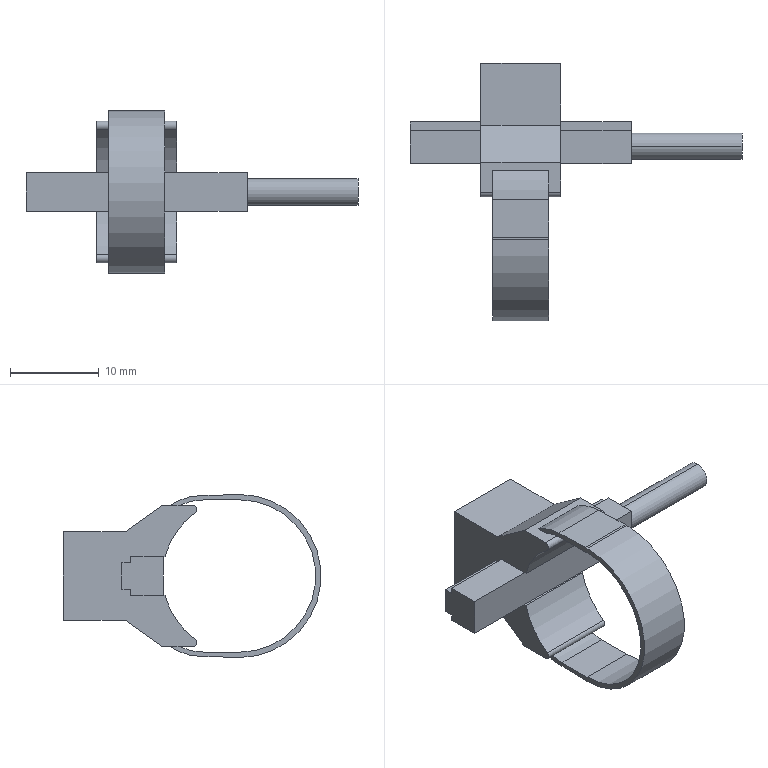Part | SolidWorks | features BaseBody 1 | 1 solid | 49 faces | box 37.5 x 29.1 x 18.4 mm | volume 1877 mm3 | plane 35 | cylinder 14 | commonest cylinder face diameters 12.4 x4 18.4 x3 1 x2 3 x2 17.4 x2 17.2 x1
STEP:
#1=CARTESIAN_POINT('',(24.,10.55,-1.5));
#2=VERTEX_POINT('',#1);
#3=CARTESIAN_POINT('',(24.,10.55,1.5));
#4=VERTEX_POINT('',#3);
#5=CARTESIAN_POINT('',(24.,10.55,0.));
#6=DIRECTION('',(-1.,0.,0.));
#7=DIRECTION('',(0.,0.,-1.));
#8=AXIS2_PLACEMENT_3D('',#5,#6,#7);
#9=CIRCLE('',#8,1.5);
#10=EDGE_CURVE('',#2,#4,#9,.T.);
#11=ORIENTED_EDGE('',*,*,#10,.F.);
#12=CARTESIAN_POINT('',(36.5,10.55,-1.5));
#13=VERTEX_POINT('',#12);
#14=CARTESIAN_POINT('',(36.5,10.55,-1.5));
#15=DIRECTION('',(1.,0.,0.));
#16=VECTOR('',#15,1000.);
#17=LINE('',#14,#16);
#18=EDGE_CURVE('',#2,#13,#17,.T.);
#19=ORIENTED_EDGE('',*,*,#18,.T.);
#20=CARTESIAN_POINT('',(36.5,10.55,1.5));
#21=VERTEX_POINT('',#20);
#22=CARTESIAN_POINT('',(36.5,10.55,0.));
#23=DIRECTION('',(1.,0.,0.));
#24=DIRECTION('',(0.,0.,-1.));
#25=AXIS2_PLACEMENT_3D('',#22,#23,#24);
#26=CIRCLE('',#25,1.5);
#27=EDGE_CURVE('',#21,#13,#26,.T.);
#28=ORIENTED_EDGE('',*,*,#27,.F.);
#29=CARTESIAN_POINT('',(36.5,10.55,1.5));
#30=DIRECTION('',(1.,0.,0.));
#31=VECTOR('',#30,1000.);
#32=LINE('',#29,#31);
#33=EDGE_CURVE('',#4,#21,#32,.T.);
#34=ORIENTED_EDGE('',*,*,#33,.F.);
#35=EDGE_LOOP('',(#11,#19,#28,#34));
#36=FACE_OUTER_BOUND('',#35,.T.);
#37=CARTESIAN_POINT('',(36.5,10.55,0.));
#38=DIRECTION('',(1.,0.,0.));
#39=DIRECTION('',(0.,0.,1.));
#40=AXIS2_PLACEMENT_3D('',#37,#38,#39);
#41=CYLINDRICAL_SURFACE('',#40,1.5);
#42=ADVANCED_FACE('',(#36),#41,.T.);
#43=CARTESIAN_POINT('',(8.325,0.,9.2));
#44=VERTEX_POINT('',#43);
#45=CARTESIAN_POINT('',(8.325,0.,-9.2));
#46=VERTEX_POINT('',#45);
#47=CARTESIAN_POINT('',(8.325,0.,0.));
#48=DIRECTION('',(1.,0.,0.));
#49=DIRECTION('',(0.,0.,-1.));
#50=AXIS2_PLACEMENT_3D('',#47,#48,#49);
#51=CIRCLE('',#50,9.2);
#52=EDGE_CURVE('',#44,#46,#51,.T.);
#53=ORIENTED_EDGE('',*,*,#52,.T.);
#54=CARTESIAN_POINT('',(14.675,0.,-9.2));
#55=VERTEX_POINT('',#54);
#56=CARTESIAN_POINT('',(14.675,0.,-9.2));
#57=DIRECTION('',(1.,0.,0.));
#58=VECTOR('',#57,1000.);
#59=LINE('',#56,#58);
#60=EDGE_CURVE('',#46,#55,#59,.T.);
#61=ORIENTED_EDGE('',*,*,#60,.T.);
#62=CARTESIAN_POINT('',(14.675,0.,9.2));
#63=VERTEX_POINT('',#62);
#64=CARTESIAN_POINT('',(14.675,0.,0.));
#65=DIRECTION('',(1.,0.,0.));
#66=DIRECTION('',(0.,0.,-1.));
#67=AXIS2_PLACEMENT_3D('',#64,#65,#66);
#68=CIRCLE('',#67,9.2);
#69=EDGE_CURVE('',#63,#55,#68,.T.);
#70=ORIENTED_EDGE('',*,*,#69,.F.);
#71=CARTESIAN_POINT('',(14.675,0.,9.2));
#72=DIRECTION('',(1.,0.,0.));
#73=VECTOR('',#72,1000.);
#74=LINE('',#71,#73);
#75=EDGE_CURVE('',#44,#63,#74,.T.);
#76=ORIENTED_EDGE('',*,*,#75,.F.);
#77=EDGE_LOOP('',(#53,#61,#70,#76));
#78=FACE_OUTER_BOUND('',#77,.T.);
#79=CARTESIAN_POINT('',(14.675,0.,0.));
#80=DIRECTION('',(1.,0.,0.));
#81=DIRECTION('',(0.,0.,1.));
#82=AXIS2_PLACEMENT_3D('',#79,#80,#81);
#83=CYLINDRICAL_SURFACE('',#82,9.2);
#84=ADVANCED_FACE('',(#78),#83,.T.);
#85=CARTESIAN_POINT('',(8.325,0.2661,9.196));
#86=VERTEX_POINT('',#85);
#87=CARTESIAN_POINT('',(8.325,0.,0.));
#88=DIRECTION('',(1.,0.,0.));
#89=DIRECTION('',(0.,0.,-1.));
#90=AXIS2_PLACEMENT_3D('',#87,#88,#89);
#91=CIRCLE('',#90,9.2);
#92=EDGE_CURVE('',#86,#44,#91,.T.);
#93=ORIENTED_EDGE('',*,*,#92,.T.);
#94=ORIENTED_EDGE('',*,*,#75,.T.);
#95=CARTESIAN_POINT('',(14.675,0.2661,9.196));
#96=VERTEX_POINT('',#95);
#97=CARTESIAN_POINT('',(14.675,0.,0.));
#98=DIRECTION('',(1.,0.,0.));
#99=DIRECTION('',(0.,0.,-1.));
#100=AXIS2_PLACEMENT_3D('',#97,#98,#99);
#101=CIRCLE('',#100,9.2);
#102=EDGE_CURVE('',#96,#63,#101,.T.);
#103=ORIENTED_EDGE('',*,*,#102,.F.);
#104=CARTESIAN_POINT('',(14.675,0.2661,9.196));
#105=DIRECTION('',(-1.,0.,0.));
#106=VECTOR('',#105,1000.);
#107=LINE('',#104,#106);
#108=EDGE_CURVE('',#96,#86,#107,.T.);
#109=ORIENTED_EDGE('',*,*,#108,.T.);
#110=EDGE_LOOP('',(#93,#94,#103,#109));
#111=FACE_OUTER_BOUND('',#110,.T.);
#112=CARTESIAN_POINT('',(14.675,0.,0.));
#113=DIRECTION('',(1.,0.,0.));
#114=DIRECTION('',(0.,0.,1.));
#115=AXIS2_PLACEMENT_3D('',#112,#113,#114);
#116=CYLINDRICAL_SURFACE('',#115,9.2);
#117=ADVANCED_FACE('',(#111),#116,.T.);
#118=CARTESIAN_POINT('',(7.,19.9,5.));
#119=VERTEX_POINT('',#118);
#120=CARTESIAN_POINT('',(7.,12.9,5.));
#121=VERTEX_POINT('',#120);
#122=CARTESIAN_POINT('',(7.,19.9,5.));
#123=DIRECTION('',(0.,-1.,0.));
#124=VECTOR('',#123,1000.);
#125=LINE('',#122,#124);
#126=EDGE_CURVE('',#119,#121,#125,.T.);
#127=ORIENTED_EDGE('',*,*,#126,.T.);
#128=CARTESIAN_POINT('',(16.,12.9,5.));
#129=VERTEX_POINT('',#128);
#130=CARTESIAN_POINT('',(16.,12.9,5.));
#131=DIRECTION('',(-1.,0.,0.));
#132=VECTOR('',#131,1000.);
#133=LINE('',#130,#132);
#134=EDGE_CURVE('',#129,#121,#133,.T.);
#135=ORIENTED_EDGE('',*,*,#134,.F.);
#136=CARTESIAN_POINT('',(16.,19.9,5.));
#137=VERTEX_POINT('',#136);
#138=CARTESIAN_POINT('',(16.,19.9,5.));
#139=DIRECTION('',(0.,-1.,0.));
#140=VECTOR('',#139,1000.);
#141=LINE('',#138,#140);
#142=EDGE_CURVE('',#137,#129,#141,.T.);
#143=ORIENTED_EDGE('',*,*,#142,.F.);
#144=CARTESIAN_POINT('',(16.,19.9,5.));
#145=DIRECTION('',(-1.,0.,0.));
#146=VECTOR('',#145,1000.);
#147=LINE('',#144,#146);
#148=EDGE_CURVE('',#137,#119,#147,.T.);
#149=ORIENTED_EDGE('',*,*,#148,.T.);
#150=EDGE_LOOP('',(#127,#135,#143,#149));
#151=FACE_OUTER_BOUND('',#150,.T.);
#152=CARTESIAN_POINT('',(16.,19.9,5.));
#153=DIRECTION('',(0.,0.,-1.));
#154=DIRECTION('',(0.,-1.,0.));
#155=AXIS2_PLACEMENT_3D('',#152,#153,#154);
#156=PLANE('',#155);
#157=ADVANCED_FACE('',(#151),#156,.F.);
#158=CARTESIAN_POINT('',(7.,19.9,-5.));
#159=VERTEX_POINT('',#158);
#160=CARTESIAN_POINT('',(7.,19.9,-5.));
#161=DIRECTION('',(0.,0.,1.));
#162=VECTOR('',#161,1000.);
#163=LINE('',#160,#162);
#164=EDGE_CURVE('',#159,#119,#163,.T.);
#165=ORIENTED_EDGE('',*,*,#164,.T.);
#166=ORIENTED_EDGE('',*,*,#148,.F.);
#167=CARTESIAN_POINT('',(16.,19.9,-5.));
#168=VERTEX_POINT('',#167);
#169=CARTESIAN_POINT('',(16.,19.9,-5.));
#170=DIRECTION('',(0.,0.,1.));
#171=VECTOR('',#170,1000.);
#172=LINE('',#169,#171);
#173=EDGE_CURVE('',#168,#137,#172,.T.);
#174=ORIENTED_EDGE('',*,*,#173,.F.);
#175=CARTESIAN_POINT('',(16.,19.9,-5.));
#176=DIRECTION('',(-1.,0.,0.));
#177=VECTOR('',#176,1000.);
#178=LINE('',#175,#177);
#179=EDGE_CURVE('',#168,#159,#178,.T.);
#180=ORIENTED_EDGE('',*,*,#179,.T.);
#181=EDGE_LOOP('',(#165,#166,#174,#180));
#182=FACE_OUTER_BOUND('',#181,.T.);
#183=CARTESIAN_POINT('',(16.,19.9,-5.));
#184=DIRECTION('',(0.,-1.,0.));
#185=DIRECTION('',(0.,0.,-1.));
#186=AXIS2_PLACEMENT_3D('',#183,#184,#185);
#187=PLANE('',#186);
#188=ADVANCED_FACE('',(#182),#187,.F.);
#189=CARTESIAN_POINT('',(7.,12.9,-5.));
#190=VERTEX_POINT('',#189);
#191=CARTESIAN_POINT('',(7.,12.9,-5.));
#192=DIRECTION('',(0.,1.,0.));
#193=VECTOR('',#192,1000.);
#194=LINE('',#191,#193);
#195=EDGE_CURVE('',#190,#159,#194,.T.);
#196=ORIENTED_EDGE('',*,*,#195,.T.);
#197=ORIENTED_EDGE('',*,*,#179,.F.);
#198=CARTESIAN_POINT('',(16.,12.9,-5.));
#199=VERTEX_POINT('',#198);
#200=CARTESIAN_POINT('',(16.,12.9,-5.));
#201=DIRECTION('',(0.,1.,0.));
#202=VECTOR('',#201,1000.);
#203=LINE('',#200,#202);
#204=EDGE_CURVE('',#199,#168,#203,.T.);
#205=ORIENTED_EDGE('',*,*,#204,.F.);
#206=CARTESIAN_POINT('',(16.,12.9,-5.));
#207=DIRECTION('',(-1.,0.,0.));
#208=VECTOR('',#207,1000.);
#209=LINE('',#206,#208);
#210=EDGE_CURVE('',#199,#190,#209,.T.);
#211=ORIENTED_EDGE('',*,*,#210,.T.);
#212=EDGE_LOOP('',(#196,#197,#205,#211));
#213=FACE_OUTER_BOUND('',#212,.T.);
#214=CARTESIAN_POINT('',(16.,12.9,-5.));
#215=DIRECTION('',(0.,0.,1.));
#216=DIRECTION('',(1.,0.,0.));
#217=AXIS2_PLACEMENT_3D('',#214,#215,#216);
#218=PLANE('',#217);
#219=ADVANCED_FACE('',(#213),#218,.F.);
#220=CARTESIAN_POINT('',(7.,5.039,-7.092));
#221=VERTEX_POINT('',#220);
#222=CARTESIAN_POINT('',(7.,8.417,-2.2));
#223=VERTEX_POINT('',#222);
#224=CARTESIAN_POINT('',(7.,0.,0.));
#225=DIRECTION('',(1.,0.,0.));
#226=DIRECTION('',(0.,0.,-1.));
#227=AXIS2_PLACEMENT_3D('',#224,#225,#226);
#228=CIRCLE('',#227,8.7);
#229=EDGE_CURVE('',#221,#223,#228,.T.);
#230=ORIENTED_EDGE('',*,*,#229,.F.);
#231=CARTESIAN_POINT('',(16.,5.039,-7.092));
#232=VERTEX_POINT('',#231);
#233=CARTESIAN_POINT('',(16.,5.039,-7.092));
#234=DIRECTION('',(-1.,0.,0.));
#235=VECTOR('',#234,1000.);
#236=LINE('',#233,#235);
#237=EDGE_CURVE('',#232,#221,#236,.T.);
#238=ORIENTED_EDGE('',*,*,#237,.F.);
#239=CARTESIAN_POINT('',(16.,8.417,-2.2));
#240=VERTEX_POINT('',#239);
#241=CARTESIAN_POINT('',(16.,0.,0.));
#242=DIRECTION('',(1.,0.,0.));
#243=DIRECTION('',(0.,0.,-1.));
#244=AXIS2_PLACEMENT_3D('',#241,#242,#243);
#245=CIRCLE('',#244,8.7);
#246=EDGE_CURVE('',#232,#240,#245,.T.);
#247=ORIENTED_EDGE('',*,*,#246,.T.);
#248=CARTESIAN_POINT('',(16.,8.417,-2.2));
#249=DIRECTION('',(-1.,0.,0.));
#250=VECTOR('',#249,1000.);
#251=LINE('',#248,#250);
#252=EDGE_CURVE('',#240,#223,#251,.T.);
#253=ORIENTED_EDGE('',*,*,#252,.T.);
#254=EDGE_LOOP('',(#230,#238,#247,#253));
#255=FACE_OUTER_BOUND('',#254,.T.);
#256=CARTESIAN_POINT('',(16.,0.,0.));
#257=DIRECTION('',(1.,0.,0.));
#258=DIRECTION('',(0.,0.,1.));
#259=AXIS2_PLACEMENT_3D('',#256,#257,#258);
#260=CYLINDRICAL_SURFACE('',#259,8.7);
#261=ADVANCED_FACE('',(#255),#260,.F.);
#262=CARTESIAN_POINT('',(7.,5.328,-8.));
#263=VERTEX_POINT('',#262);
#264=CARTESIAN_POINT('',(7.,5.328,-7.5));
#265=DIRECTION('',(1.,0.,0.));
#266=DIRECTION('',(0.,0.,-1.));
#267=AXIS2_PLACEMENT_3D('',#264,#265,#266);
#268=CIRCLE('',#267,0.5);
#269=EDGE_CURVE('',#221,#263,#268,.T.);
#270=ORIENTED_EDGE('',*,*,#269,.T.);
#271=CARTESIAN_POINT('',(16.,5.328,-8.));
#272=VERTEX_POINT('',#271);
#273=CARTESIAN_POINT('',(16.,5.328,-8.));
#274=DIRECTION('',(-1.,0.,0.));
#275=VECTOR('',#274,1000.);
#276=LINE('',#273,#275);
#277=EDGE_CURVE('',#272,#263,#276,.T.);
#278=ORIENTED_EDGE('',*,*,#277,.F.);
#279=CARTESIAN_POINT('',(16.,5.328,-7.5));
#280=DIRECTION('',(1.,0.,0.));
#281=DIRECTION('',(0.,0.,-1.));
#282=AXIS2_PLACEMENT_3D('',#279,#280,#281);
#283=CIRCLE('',#282,0.5);
#284=EDGE_CURVE('',#232,#272,#283,.T.);
#285=ORIENTED_EDGE('',*,*,#284,.F.);
#286=ORIENTED_EDGE('',*,*,#237,.T.);
#287=EDGE_LOOP('',(#270,#278,#285,#286));
#288=FACE_OUTER_BOUND('',#287,.T.);
#289=CARTESIAN_POINT('',(16.,5.328,-7.5));
#290=DIRECTION('',(1.,0.,0.));
#291=DIRECTION('',(0.,0.,1.));
#292=AXIS2_PLACEMENT_3D('',#289,#290,#291);
#293=CYLINDRICAL_SURFACE('',#292,0.5);
#294=ADVANCED_FACE('',(#288),#293,.T.);
#295=CARTESIAN_POINT('',(7.,8.7,-8.));
#296=VERTEX_POINT('',#295);
#297=CARTESIAN_POINT('',(7.,8.7,-8.));
#298=DIRECTION('',(0.,0.8137,0.5812));
#299=VECTOR('',#298,1000.);
#300=LINE('',#297,#299);
#301=EDGE_CURVE('',#296,#190,#300,.T.);
#302=ORIENTED_EDGE('',*,*,#301,.T.);
#303=ORIENTED_EDGE('',*,*,#210,.F.);
#304=CARTESIAN_POINT('',(16.,8.7,-8.));
#305=VERTEX_POINT('',#304);
#306=CARTESIAN_POINT('',(16.,8.7,-8.));
#307=DIRECTION('',(0.,0.8137,0.5812));
#308=VECTOR('',#307,1000.);
#309=LINE('',#306,#308);
#310=EDGE_CURVE('',#305,#199,#309,.T.);
#311=ORIENTED_EDGE('',*,*,#310,.F.);
#312=CARTESIAN_POINT('',(16.,8.7,-8.));
#313=DIRECTION('',(-1.,0.,0.));
#314=VECTOR('',#313,1000.);
#315=LINE('',#312,#314);
#316=EDGE_CURVE('',#305,#296,#315,.T.);
#317=ORIENTED_EDGE('',*,*,#316,.T.);
#318=EDGE_LOOP('',(#302,#303,#311,#317));
#319=FACE_OUTER_BOUND('',#318,.T.);
#320=CARTESIAN_POINT('',(16.,8.7,-8.));
#321=DIRECTION('',(0.,-0.5812,0.8137));
#322=DIRECTION('',(-1.,0.,0.));
#323=AXIS2_PLACEMENT_3D('',#320,#321,#322);
#324=PLANE('',#323);
#325=ADVANCED_FACE('',(#319),#324,.F.);
#326=CARTESIAN_POINT('',(8.325,6.661,-8.));
#327=VERTEX_POINT('',#326);
#328=CARTESIAN_POINT('',(14.675,6.661,-8.));
#329=VERTEX_POINT('',#328);
#330=CARTESIAN_POINT('',(14.675,6.661,-8.));
#331=DIRECTION('',(1.,0.,0.));
#332=VECTOR('',#331,1000.);
#333=LINE('',#330,#332);
#334=EDGE_CURVE('',#327,#329,#333,.T.);
#335=ORIENTED_EDGE('',*,*,#334,.T.);
#336=CARTESIAN_POINT('',(14.675,7.792,-8.));
#337=VERTEX_POINT('',#336);
#338=CARTESIAN_POINT('',(14.675,5.328,-8.));
#339=DIRECTION('',(0.,1.,0.));
#340=VECTOR('',#339,1000.);
#341=LINE('',#338,#340);
#342=EDGE_CURVE('',#329,#337,#341,.T.);
#343=ORIENTED_EDGE('',*,*,#342,.T.);
#344=CARTESIAN_POINT('',(8.325,7.792,-8.));
#345=VERTEX_POINT('',#344);
#346=CARTESIAN_POINT('',(14.675,7.792,-8.));
#347=DIRECTION('',(1.,0.,0.));
#348=VECTOR('',#347,1000.);
#349=LINE('',#346,#348);
#350=EDGE_CURVE('',#345,#337,#349,.T.);
#351=ORIENTED_EDGE('',*,*,#350,.F.);
#352=CARTESIAN_POINT('',(8.325,5.328,-8.));
#353=DIRECTION('',(0.,1.,0.));
#354=VECTOR('',#353,1000.);
#355=LINE('',#352,#354);
#356=EDGE_CURVE('',#327,#345,#355,.T.);
#357=ORIENTED_EDGE('',*,*,#356,.F.);
#358=EDGE_LOOP('',(#335,#343,#351,#357));
#359=FACE_BOUND('',#358,.T.);
#360=CARTESIAN_POINT('',(7.,5.328,-8.));
#361=DIRECTION('',(0.,1.,0.));
#362=VECTOR('',#361,1000.);
#363=LINE('',#360,#362);
#364=EDGE_CURVE('',#263,#296,#363,.T.);
#365=ORIENTED_EDGE('',*,*,#364,.T.);
#366=ORIENTED_EDGE('',*,*,#316,.F.);
#367=CARTESIAN_POINT('',(16.,5.328,-8.));
#368=DIRECTION('',(0.,1.,0.));
#369=VECTOR('',#368,1000.);
#370=LINE('',#367,#369);
#371=EDGE_CURVE('',#272,#305,#370,.T.);
#372=ORIENTED_EDGE('',*,*,#371,.F.);
#373=ORIENTED_EDGE('',*,*,#277,.T.);
#374=EDGE_LOOP('',(#365,#366,#372,#373));
#375=FACE_OUTER_BOUND('',#374,.T.);
#376=CARTESIAN_POINT('',(16.,5.328,-8.));
#377=DIRECTION('',(0.,0.,1.));
#378=DIRECTION('',(1.,0.,0.));
#379=AXIS2_PLACEMENT_3D('',#376,#377,#378);
#380=PLANE('',#379);
#381=ADVANCED_FACE('',(#359,#375),#380,.F.);
#382=CARTESIAN_POINT('',(8.325,4.479,9.074));
#383=VERTEX_POINT('',#382);
#384=CARTESIAN_POINT('',(8.325,4.479,9.074));
#385=DIRECTION('',(0.,-0.9996,0.02893));
#386=VECTOR('',#385,1000.);
#387=LINE('',#384,#386);
#388=EDGE_CURVE('',#383,#86,#387,.T.);
#389=ORIENTED_EDGE('',*,*,#388,.T.);
#390=ORIENTED_EDGE('',*,*,#108,.F.);
#391=CARTESIAN_POINT('',(14.675,4.479,9.074));
#392=VERTEX_POINT('',#391);
#393=CARTESIAN_POINT('',(14.675,4.479,9.074));
#394=DIRECTION('',(0.,-0.9996,0.02893));
#395=VECTOR('',#394,1000.);
#396=LINE('',#393,#395);
#397=EDGE_CURVE('',#392,#96,#396,.T.);
#398=ORIENTED_EDGE('',*,*,#397,.F.);
#399=CARTESIAN_POINT('',(14.675,4.479,9.074));
#400=DIRECTION('',(-1.,0.,0.));
#401=VECTOR('',#400,1000.);
#402=LINE('',#399,#401);
#403=EDGE_CURVE('',#392,#383,#402,.T.);
#404=ORIENTED_EDGE('',*,*,#403,.T.);
#405=EDGE_LOOP('',(#389,#390,#398,#404));
#406=FACE_OUTER_BOUND('',#405,.T.);
#407=CARTESIAN_POINT('',(14.675,4.479,9.074));
#408=DIRECTION('',(0.,-0.02893,-0.9996));
#409=DIRECTION('',(0.,-0.9996,0.02893));
#410=AXIS2_PLACEMENT_3D('',#407,#408,#409);
#411=PLANE('',#410);
#412=ADVANCED_FACE('',(#406),#411,.F.);
#413=ORIENTED_EDGE('',*,*,#60,.F.);
#414=CARTESIAN_POINT('',(8.325,0.2661,-9.196));
#415=VERTEX_POINT('',#414);
#416=CARTESIAN_POINT('',(8.325,0.,0.));
#417=DIRECTION('',(1.,0.,0.));
#418=DIRECTION('',(0.,0.,-1.));
#419=AXIS2_PLACEMENT_3D('',#416,#417,#418);
#420=CIRCLE('',#419,9.2);
#421=EDGE_CURVE('',#46,#415,#420,.T.);
#422=ORIENTED_EDGE('',*,*,#421,.T.);
#423=CARTESIAN_POINT('',(14.675,0.2661,-9.196));
#424=VERTEX_POINT('',#423);
#425=CARTESIAN_POINT('',(14.675,0.2661,-9.196));
#426=DIRECTION('',(-1.,0.,0.));
#427=VECTOR('',#426,1000.);
#428=LINE('',#425,#427);
#429=EDGE_CURVE('',#424,#415,#428,.T.);
#430=ORIENTED_EDGE('',*,*,#429,.F.);
#431=CARTESIAN_POINT('',(14.675,0.,0.));
#432=DIRECTION('',(1.,0.,0.));
#433=DIRECTION('',(0.,0.,-1.));
#434=AXIS2_PLACEMENT_3D('',#431,#432,#433);
#435=CIRCLE('',#434,9.2);
#436=EDGE_CURVE('',#55,#424,#435,.T.);
#437=ORIENTED_EDGE('',*,*,#436,.F.);
#438=EDGE_LOOP('',(#413,#422,#430,#437));
#439=FACE_OUTER_BOUND('',#438,.T.);
#440=CARTESIAN_POINT('',(14.675,0.,0.));
#441=DIRECTION('',(1.,0.,0.));
#442=DIRECTION('',(0.,0.,1.));
#443=AXIS2_PLACEMENT_3D('',#440,#441,#442);
#444=CYLINDRICAL_SURFACE('',#443,9.2);
#445=ADVANCED_FACE('',(#439),#444,.T.);
#446=CARTESIAN_POINT('',(8.325,4.479,-9.074));
#447=VERTEX_POINT('',#446);
#448=CARTESIAN_POINT('',(8.325,0.2661,-9.196));
#449=DIRECTION('',(0.,0.9996,0.02893));
#450=VECTOR('',#449,1000.);
#451=LINE('',#448,#450);
#452=EDGE_CURVE('',#415,#447,#451,.T.);
#453=ORIENTED_EDGE('',*,*,#452,.T.);
#454=CARTESIAN_POINT('',(14.675,4.479,-9.074));
#455=VERTEX_POINT('',#454);
#456=CARTESIAN_POINT('',(14.675,4.479,-9.074));
#457=DIRECTION('',(-1.,0.,0.));
#458=VECTOR('',#457,1000.);
#459=LINE('',#456,#458);
#460=EDGE_CURVE('',#455,#447,#459,.T.);
#461=ORIENTED_EDGE('',*,*,#460,.F.);
#462=CARTESIAN_POINT('',(14.675,0.2661,-9.196));
#463=DIRECTION('',(0.,0.9996,0.02893));
#464=VECTOR('',#463,1000.);
#465=LINE('',#462,#464);
#466=EDGE_CURVE('',#424,#455,#465,.T.);
#467=ORIENTED_EDGE('',*,*,#466,.F.);
#468=ORIENTED_EDGE('',*,*,#429,.T.);
#469=EDGE_LOOP('',(#453,#461,#467,#468));
#470=FACE_OUTER_BOUND('',#469,.T.);
#471=CARTESIAN_POINT('',(14.675,0.2661,-9.196));
#472=DIRECTION('',(0.,-0.02893,0.9996));
#473=DIRECTION('',(-1.,0.,0.));
#474=AXIS2_PLACEMENT_3D('',#471,#472,#473);
#475=PLANE('',#474);
#476=ADVANCED_FACE('',(#470),#475,.F.);
#477=CARTESIAN_POINT('',(8.325,4.3,-2.877));
#478=DIRECTION('',(1.,0.,0.));
#479=DIRECTION('',(0.,0.,-1.));
#480=AXIS2_PLACEMENT_3D('',#477,#478,#479);
#481=CIRCLE('',#480,6.2);
#482=EDGE_CURVE('',#447,#345,#481,.T.);
#483=ORIENTED_EDGE('',*,*,#482,.T.);
#484=ORIENTED_EDGE('',*,*,#350,.T.);
#485=CARTESIAN_POINT('',(14.675,4.3,-2.877));
#486=DIRECTION('',(1.,0.,0.));
#487=DIRECTION('',(0.,0.,-1.));
#488=AXIS2_PLACEMENT_3D('',#485,#486,#487);
#489=CIRCLE('',#488,6.2);
#490=EDGE_CURVE('',#455,#337,#489,.T.);
#491=ORIENTED_EDGE('',*,*,#490,.F.);
#492=ORIENTED_EDGE('',*,*,#460,.T.);
#493=EDGE_LOOP('',(#483,#484,#491,#492));
#494=FACE_OUTER_BOUND('',#493,.T.);
#495=CARTESIAN_POINT('',(14.675,4.3,-2.877));
#496=DIRECTION('',(1.,0.,0.));
#497=DIRECTION('',(0.,0.,1.));
#498=AXIS2_PLACEMENT_3D('',#495,#496,#497);
#499=CYLINDRICAL_SURFACE('',#498,6.2);
#500=ADVANCED_FACE('',(#494),#499,.T.);
#501=CARTESIAN_POINT('',(14.675,7.792,8.));
#502=VERTEX_POINT('',#501);
#503=CARTESIAN_POINT('',(14.675,4.3,2.877));
#504=DIRECTION('',(1.,0.,0.));
#505=DIRECTION('',(0.,0.,-1.));
#506=AXIS2_PLACEMENT_3D('',#503,#504,#505);
#507=CIRCLE('',#506,6.2);
#508=EDGE_CURVE('',#502,#392,#507,.T.);
#509=ORIENTED_EDGE('',*,*,#508,.F.);
#510=CARTESIAN_POINT('',(8.325,7.792,8.));
#511=VERTEX_POINT('',#510);
#512=CARTESIAN_POINT('',(14.675,7.792,8.));
#513=DIRECTION('',(-1.,0.,0.));
#514=VECTOR('',#513,1000.);
#515=LINE('',#512,#514);
#516=EDGE_CURVE('',#502,#511,#515,.T.);
#517=ORIENTED_EDGE('',*,*,#516,.T.);
#518=CARTESIAN_POINT('',(8.325,4.3,2.877));
#519=DIRECTION('',(1.,0.,0.));
#520=DIRECTION('',(0.,0.,-1.));
#521=AXIS2_PLACEMENT_3D('',#518,#519,#520);
#522=CIRCLE('',#521,6.2);
#523=EDGE_CURVE('',#511,#383,#522,.T.);
#524=ORIENTED_EDGE('',*,*,#523,.T.);
#525=ORIENTED_EDGE('',*,*,#403,.F.);
#526=EDGE_LOOP('',(#509,#517,#524,#525));
#527=FACE_OUTER_BOUND('',#526,.T.);
#528=CARTESIAN_POINT('',(14.675,4.3,2.877));
#529=DIRECTION('',(1.,0.,0.));
#530=DIRECTION('',(0.,0.,1.));
#531=AXIS2_PLACEMENT_3D('',#528,#529,#530);
#532=CYLINDRICAL_SURFACE('',#531,6.2);
#533=ADVANCED_FACE('',(#527),#532,.T.);
#534=CARTESIAN_POINT('',(8.325,0.,8.6));
#535=VERTEX_POINT('',#534);
#536=CARTESIAN_POINT('',(8.325,0.,-8.6));
#537=VERTEX_POINT('',#536);
#538=CARTESIAN_POINT('',(8.325,0.,0.));
#539=DIRECTION('',(1.,0.,0.));
#540=DIRECTION('',(0.,0.,-1.));
#541=AXIS2_PLACEMENT_3D('',#538,#539,#540);
#542=CIRCLE('',#541,8.6);
#543=EDGE_CURVE('',#535,#537,#542,.T.);
#544=ORIENTED_EDGE('',*,*,#543,.F.);
#545=CARTESIAN_POINT('',(14.675,0.,8.6));
#546=VERTEX_POINT('',#545);
#547=CARTESIAN_POINT('',(14.675,0.,8.6));
#548=DIRECTION('',(-1.,0.,0.));
#549=VECTOR('',#548,1000.);
#550=LINE('',#547,#549);
#551=EDGE_CURVE('',#546,#535,#550,.T.);
#552=ORIENTED_EDGE('',*,*,#551,.F.);
#553=CARTESIAN_POINT('',(14.675,0.,-8.6));
#554=VERTEX_POINT('',#553);
#555=CARTESIAN_POINT('',(14.675,0.,0.));
#556=DIRECTION('',(1.,0.,0.));
#557=DIRECTION('',(0.,0.,-1.));
#558=AXIS2_PLACEMENT_3D('',#555,#556,#557);
#559=CIRCLE('',#558,8.6);
#560=EDGE_CURVE('',#546,#554,#559,.T.);
#561=ORIENTED_EDGE('',*,*,#560,.T.);
#562=CARTESIAN_POINT('',(14.675,0.,-8.6));
#563=DIRECTION('',(-1.,0.,0.));
#564=VECTOR('',#563,1000.);
#565=LINE('',#562,#564);
#566=EDGE_CURVE('',#554,#537,#565,.T.);
#567=ORIENTED_EDGE('',*,*,#566,.T.);
#568=EDGE_LOOP('',(#544,#552,#561,#567));
#569=FACE_OUTER_BOUND('',#568,.T.);
#570=CARTESIAN_POINT('',(14.675,0.,0.));
#571=DIRECTION('',(1.,0.,0.));
#572=DIRECTION('',(0.,0.,1.));
#573=AXIS2_PLACEMENT_3D('',#570,#571,#572);
#574=CYLINDRICAL_SURFACE('',#573,8.6);
#575=ADVANCED_FACE('',(#569),#574,.F.);
#576=CARTESIAN_POINT('',(8.325,4.,-8.6));
#577=VERTEX_POINT('',#576);
#578=CARTESIAN_POINT('',(8.325,0.,-8.6));
#579=DIRECTION('',(0.,1.,0.));
#580=VECTOR('',#579,1000.);
#581=LINE('',#578,#580);
#582=EDGE_CURVE('',#537,#577,#581,.T.);
#583=ORIENTED_EDGE('',*,*,#582,.F.);
#584=ORIENTED_EDGE('',*,*,#566,.F.);
#585=CARTESIAN_POINT('',(14.675,4.,-8.6));
#586=VERTEX_POINT('',#585);
#587=CARTESIAN_POINT('',(14.675,0.,-8.6));
#588=DIRECTION('',(0.,1.,0.));
#589=VECTOR('',#588,1000.);
#590=LINE('',#587,#589);
#591=EDGE_CURVE('',#554,#586,#590,.T.);
#592=ORIENTED_EDGE('',*,*,#591,.T.);
#593=CARTESIAN_POINT('',(14.675,4.,-8.6));
#594=DIRECTION('',(-1.,0.,0.));
#595=VECTOR('',#594,1000.);
#596=LINE('',#593,#595);
#597=EDGE_CURVE('',#586,#577,#596,.T.);
#598=ORIENTED_EDGE('',*,*,#597,.T.);
#599=EDGE_LOOP('',(#583,#584,#592,#598));
#600=FACE_OUTER_BOUND('',#599,.T.);
#601=CARTESIAN_POINT('',(14.675,0.,-8.6));
#602=DIRECTION('',(0.,0.,1.));
#603=DIRECTION('',(0.,-1.,0.));
#604=AXIS2_PLACEMENT_3D('',#601,#602,#603);
#605=PLANE('',#604);
#606=ADVANCED_FACE('',(#600),#605,.T.);
#607=ORIENTED_EDGE('',*,*,#334,.F.);
#608=CARTESIAN_POINT('',(8.325,4.,-2.4));
#609=DIRECTION('',(1.,0.,0.));
#610=DIRECTION('',(0.,0.,-1.));
#611=AXIS2_PLACEMENT_3D('',#608,#609,#610);
#612=CIRCLE('',#611,6.2);
#613=EDGE_CURVE('',#577,#327,#612,.T.);
#614=ORIENTED_EDGE('',*,*,#613,.F.);
#615=ORIENTED_EDGE('',*,*,#597,.F.);
#616=CARTESIAN_POINT('',(14.675,4.,-2.4));
#617=DIRECTION('',(1.,0.,0.));
#618=DIRECTION('',(0.,0.,-1.));
#619=AXIS2_PLACEMENT_3D('',#616,#617,#618);
#620=CIRCLE('',#619,6.2);
#621=EDGE_CURVE('',#586,#329,#620,.T.);
#622=ORIENTED_EDGE('',*,*,#621,.T.);
#623=EDGE_LOOP('',(#607,#614,#615,#622));
#624=FACE_OUTER_BOUND('',#623,.T.);
#625=CARTESIAN_POINT('',(14.675,4.,-2.4));
#626=DIRECTION('',(1.,0.,0.));
#627=DIRECTION('',(0.,0.,1.));
#628=AXIS2_PLACEMENT_3D('',#625,#626,#627);
#629=CYLINDRICAL_SURFACE('',#628,6.2);
#630=ADVANCED_FACE('',(#624),#629,.F.);
#631=CARTESIAN_POINT('',(8.325,4.,8.6));
#632=VERTEX_POINT('',#631);
#633=CARTESIAN_POINT('',(8.325,4.,8.6));
#634=DIRECTION('',(0.,-1.,0.));
#635=VECTOR('',#634,1000.);
#636=LINE('',#633,#635);
#637=EDGE_CURVE('',#632,#535,#636,.T.);
#638=ORIENTED_EDGE('',*,*,#637,.F.);
#639=CARTESIAN_POINT('',(14.675,4.,8.6));
#640=VERTEX_POINT('',#639);
#641=CARTESIAN_POINT('',(14.675,4.,8.6));
#642=DIRECTION('',(-1.,0.,0.));
#643=VECTOR('',#642,1000.);
#644=LINE('',#641,#643);
#645=EDGE_CURVE('',#640,#632,#644,.T.);
#646=ORIENTED_EDGE('',*,*,#645,.F.);
#647=CARTESIAN_POINT('',(14.675,4.,8.6));
#648=DIRECTION('',(0.,-1.,0.));
#649=VECTOR('',#648,1000.);
#650=LINE('',#647,#649);
#651=EDGE_CURVE('',#640,#546,#650,.T.);
#652=ORIENTED_EDGE('',*,*,#651,.T.);
#653=ORIENTED_EDGE('',*,*,#551,.T.);
#654=EDGE_LOOP('',(#638,#646,#652,#653));
#655=FACE_OUTER_BOUND('',#654,.T.);
#656=CARTESIAN_POINT('',(14.675,4.,8.6));
#657=DIRECTION('',(0.,0.,-1.));
#658=DIRECTION('',(0.,-1.,0.));
#659=AXIS2_PLACEMENT_3D('',#656,#657,#658);
#660=PLANE('',#659);
#661=ADVANCED_FACE('',(#655),#660,.T.);
#662=ORIENTED_EDGE('',*,*,#523,.F.);
#663=CARTESIAN_POINT('',(8.325,6.661,8.));
#664=VERTEX_POINT('',#663);
#665=CARTESIAN_POINT('',(8.325,8.7,8.));
#666=DIRECTION('',(0.,-1.,0.));
#667=VECTOR('',#666,1000.);
#668=LINE('',#665,#667);
#669=EDGE_CURVE('',#511,#664,#668,.T.);
#670=ORIENTED_EDGE('',*,*,#669,.T.);
#671=CARTESIAN_POINT('',(8.325,4.,2.4));
#672=DIRECTION('',(1.,0.,0.));
#673=DIRECTION('',(0.,0.,-1.));
#674=AXIS2_PLACEMENT_3D('',#671,#672,#673);
#675=CIRCLE('',#674,6.2);
#676=EDGE_CURVE('',#664,#632,#675,.T.);
#677=ORIENTED_EDGE('',*,*,#676,.T.);
#678=ORIENTED_EDGE('',*,*,#637,.T.);
#679=ORIENTED_EDGE('',*,*,#543,.T.);
#680=ORIENTED_EDGE('',*,*,#582,.T.);
#681=ORIENTED_EDGE('',*,*,#613,.T.);
#682=ORIENTED_EDGE('',*,*,#356,.T.);
#683=ORIENTED_EDGE('',*,*,#482,.F.);
#684=ORIENTED_EDGE('',*,*,#452,.F.);
#685=ORIENTED_EDGE('',*,*,#421,.F.);
#686=ORIENTED_EDGE('',*,*,#52,.F.);
#687=ORIENTED_EDGE('',*,*,#92,.F.);
#688=ORIENTED_EDGE('',*,*,#388,.F.);
#689=EDGE_LOOP('',(#662,#670,#677,#678,#679,#680,#681,#682,#683,#684,#685,#686,#687,#688));
#690=FACE_OUTER_BOUND('',#689,.T.);
#691=CARTESIAN_POINT('',(8.325,0.,0.));
#692=DIRECTION('',(1.,0.,0.));
#693=DIRECTION('',(0.,1.,0.));
#694=AXIS2_PLACEMENT_3D('',#691,#692,#693);
#695=PLANE('',#694);
#696=ADVANCED_FACE('',(#690),#695,.F.);
#697=CARTESIAN_POINT('',(14.675,6.661,8.));
#698=VERTEX_POINT('',#697);
#699=CARTESIAN_POINT('',(14.675,8.7,8.));
#700=DIRECTION('',(0.,-1.,0.));
#701=VECTOR('',#700,1000.);
#702=LINE('',#699,#701);
#703=EDGE_CURVE('',#502,#698,#702,.T.);
#704=ORIENTED_EDGE('',*,*,#703,.F.);
#705=ORIENTED_EDGE('',*,*,#508,.T.);
#706=ORIENTED_EDGE('',*,*,#397,.T.);
#707=ORIENTED_EDGE('',*,*,#102,.T.);
#708=ORIENTED_EDGE('',*,*,#69,.T.);
#709=ORIENTED_EDGE('',*,*,#436,.T.);
#710=ORIENTED_EDGE('',*,*,#466,.T.);
#711=ORIENTED_EDGE('',*,*,#490,.T.);
#712=ORIENTED_EDGE('',*,*,#342,.F.);
#713=ORIENTED_EDGE('',*,*,#621,.F.);
#714=ORIENTED_EDGE('',*,*,#591,.F.);
#715=ORIENTED_EDGE('',*,*,#560,.F.);
#716=ORIENTED_EDGE('',*,*,#651,.F.);
#717=CARTESIAN_POINT('',(14.675,4.,2.4));
#718=DIRECTION('',(1.,0.,0.));
#719=DIRECTION('',(0.,0.,-1.));
#720=AXIS2_PLACEMENT_3D('',#717,#718,#719);
#721=CIRCLE('',#720,6.2);
#722=EDGE_CURVE('',#698,#640,#721,.T.);
#723=ORIENTED_EDGE('',*,*,#722,.F.);
#724=EDGE_LOOP('',(#704,#705,#706,#707,#708,#709,#710,#711,#712,#713,#714,#715,#716,#723));
#725=FACE_OUTER_BOUND('',#724,.T.);
#726=CARTESIAN_POINT('',(14.675,0.,0.));
#727=DIRECTION('',(1.,0.,0.));
#728=DIRECTION('',(0.,1.,0.));
#729=AXIS2_PLACEMENT_3D('',#726,#727,#728);
#730=PLANE('',#729);
#731=ADVANCED_FACE('',(#725),#730,.T.);
#732=CARTESIAN_POINT('',(7.,13.3,-1.5));
#733=VERTEX_POINT('',#732);
#734=CARTESIAN_POINT('',(-1.,13.3,-1.5));
#735=VERTEX_POINT('',#734);
#736=CARTESIAN_POINT('',(24.,13.3,-1.5));
#737=DIRECTION('',(-1.,0.,0.));
#738=VECTOR('',#737,1000.);
#739=LINE('',#736,#738);
#740=EDGE_CURVE('',#733,#735,#739,.T.);
#741=ORIENTED_EDGE('',*,*,#740,.F.);
#742=CARTESIAN_POINT('',(7.,12.3,-1.5));
#743=VERTEX_POINT('',#742);
#744=CARTESIAN_POINT('',(7.,12.9,-1.5));
#745=DIRECTION('',(0.,-1.,0.));
#746=VECTOR('',#745,1000.);
#747=LINE('',#744,#746);
#748=EDGE_CURVE('',#733,#743,#747,.T.);
#749=ORIENTED_EDGE('',*,*,#748,.T.);
#750=CARTESIAN_POINT('',(-1.,12.3,-1.5));
#751=VERTEX_POINT('',#750);
#752=CARTESIAN_POINT('',(24.,12.3,-1.5));
#753=DIRECTION('',(-1.,0.,0.));
#754=VECTOR('',#753,1000.);
#755=LINE('',#752,#754);
#756=EDGE_CURVE('',#743,#751,#755,.T.);
#757=ORIENTED_EDGE('',*,*,#756,.T.);
#758=CARTESIAN_POINT('',(-1.,12.3,-1.5));
#759=DIRECTION('',(0.,1.,0.));
#760=VECTOR('',#759,1000.);
#761=LINE('',#758,#760);
#762=EDGE_CURVE('',#751,#735,#761,.T.);
#763=ORIENTED_EDGE('',*,*,#762,.T.);
#764=EDGE_LOOP('',(#741,#749,#757,#763));
#765=FACE_OUTER_BOUND('',#764,.T.);
#766=CARTESIAN_POINT('',(24.,12.3,-1.5));
#767=DIRECTION('',(0.,0.,1.));
#768=DIRECTION('',(0.,-1.,0.));
#769=AXIS2_PLACEMENT_3D('',#766,#767,#768);
#770=PLANE('',#769);
#771=ADVANCED_FACE('',(#765),#770,.F.);
#772=CARTESIAN_POINT('',(7.,13.3,1.5));
#773=VERTEX_POINT('',#772);
#774=CARTESIAN_POINT('',(-1.,13.3,1.5));
#775=VERTEX_POINT('',#774);
#776=CARTESIAN_POINT('',(24.,13.3,1.5));
#777=DIRECTION('',(-1.,0.,0.));
#778=VECTOR('',#777,1000.);
#779=LINE('',#776,#778);
#780=EDGE_CURVE('',#773,#775,#779,.T.);
#781=ORIENTED_EDGE('',*,*,#780,.F.);
#782=CARTESIAN_POINT('',(7.,13.3,7.5));
#783=DIRECTION('',(0.,0.,-1.));
#784=VECTOR('',#783,1000.);
#785=LINE('',#782,#784);
#786=EDGE_CURVE('',#773,#733,#785,.T.);
#787=ORIENTED_EDGE('',*,*,#786,.T.);
#788=ORIENTED_EDGE('',*,*,#740,.T.);
#789=CARTESIAN_POINT('',(-1.,13.3,-1.5));
#790=DIRECTION('',(0.,0.,1.));
#791=VECTOR('',#790,1000.);
#792=LINE('',#789,#791);
#793=EDGE_CURVE('',#735,#775,#792,.T.);
#794=ORIENTED_EDGE('',*,*,#793,.T.);
#795=EDGE_LOOP('',(#781,#787,#788,#794));
#796=FACE_OUTER_BOUND('',#795,.T.);
#797=CARTESIAN_POINT('',(24.,13.3,-1.5));
#798=DIRECTION('',(0.,-1.,0.));
#799=DIRECTION('',(0.,0.,-1.));
#800=AXIS2_PLACEMENT_3D('',#797,#798,#799);
#801=PLANE('',#800);
#802=ADVANCED_FACE('',(#796),#801,.F.);
#803=CARTESIAN_POINT('',(7.,12.3,1.5));
#804=VERTEX_POINT('',#803);
#805=CARTESIAN_POINT('',(-1.,12.3,1.5));
#806=VERTEX_POINT('',#805);
#807=CARTESIAN_POINT('',(24.,12.3,1.5));
#808=DIRECTION('',(-1.,0.,0.));
#809=VECTOR('',#808,1000.);
#810=LINE('',#807,#809);
#811=EDGE_CURVE('',#804,#806,#810,.T.);
#812=ORIENTED_EDGE('',*,*,#811,.F.);
#813=CARTESIAN_POINT('',(7.,11.9,1.5));
#814=DIRECTION('',(0.,1.,0.));
#815=VECTOR('',#814,1000.);
#816=LINE('',#813,#815);
#817=EDGE_CURVE('',#804,#773,#816,.T.);
#818=ORIENTED_EDGE('',*,*,#817,.T.);
#819=ORIENTED_EDGE('',*,*,#780,.T.);
#820=CARTESIAN_POINT('',(-1.,13.3,1.5));
#821=DIRECTION('',(0.,-1.,0.));
#822=VECTOR('',#821,1000.);
#823=LINE('',#820,#822);
#824=EDGE_CURVE('',#775,#806,#823,.T.);
#825=ORIENTED_EDGE('',*,*,#824,.T.);
#826=EDGE_LOOP('',(#812,#818,#819,#825));
#827=FACE_OUTER_BOUND('',#826,.T.);
#828=CARTESIAN_POINT('',(24.,13.3,1.5));
#829=DIRECTION('',(0.,0.,-1.));
#830=DIRECTION('',(0.,-1.,0.));
#831=AXIS2_PLACEMENT_3D('',#828,#829,#830);
#832=PLANE('',#831);
#833=ADVANCED_FACE('',(#827),#832,.F.);
#834=ORIENTED_EDGE('',*,*,#27,.T.);
#835=CARTESIAN_POINT('',(36.5,10.55,0.));
#836=DIRECTION('',(1.,0.,0.));
#837=DIRECTION('',(0.,0.,-1.));
#838=AXIS2_PLACEMENT_3D('',#835,#836,#837);
#839=CIRCLE('',#838,1.5);
#840=EDGE_CURVE('',#13,#21,#839,.T.);
#841=ORIENTED_EDGE('',*,*,#840,.T.);
#842=EDGE_LOOP('',(#834,#841));
#843=FACE_OUTER_BOUND('',#842,.T.);
#844=CARTESIAN_POINT('',(36.5,10.55,0.));
#845=DIRECTION('',(1.,0.,0.));
#846=DIRECTION('',(0.,1.,0.));
#847=AXIS2_PLACEMENT_3D('',#844,#845,#846);
#848=PLANE('',#847);
#849=ADVANCED_FACE('',(#843),#848,.T.);
#850=ORIENTED_EDGE('',*,*,#18,.F.);
#851=CARTESIAN_POINT('',(24.,10.55,0.));
#852=DIRECTION('',(-1.,0.,0.));
#853=DIRECTION('',(0.,0.,-1.));
#854=AXIS2_PLACEMENT_3D('',#851,#852,#853);
#855=CIRCLE('',#854,1.5);
#856=EDGE_CURVE('',#4,#2,#855,.T.);
#857=ORIENTED_EDGE('',*,*,#856,.F.);
#858=ORIENTED_EDGE('',*,*,#33,.T.);
#859=ORIENTED_EDGE('',*,*,#840,.F.);
#860=EDGE_LOOP('',(#850,#857,#858,#859));
#861=FACE_OUTER_BOUND('',#860,.T.);
#862=CARTESIAN_POINT('',(36.5,10.55,0.));
#863=DIRECTION('',(1.,0.,0.));
#864=DIRECTION('',(0.,0.,1.));
#865=AXIS2_PLACEMENT_3D('',#862,#863,#864);
#866=CYLINDRICAL_SURFACE('',#865,1.5);
#867=ADVANCED_FACE('',(#861),#866,.T.);
#868=ORIENTED_EDGE('',*,*,#856,.T.);
#869=ORIENTED_EDGE('',*,*,#10,.T.);
#870=EDGE_LOOP('',(#868,#869));
#871=FACE_BOUND('',#870,.T.);
#872=CARTESIAN_POINT('',(24.,12.3,1.5));
#873=VERTEX_POINT('',#872);
#874=CARTESIAN_POINT('',(24.,12.3,2.2));
#875=VERTEX_POINT('',#874);
#876=CARTESIAN_POINT('',(24.,12.3,1.5));
#877=DIRECTION('',(0.,0.,1.));
#878=VECTOR('',#877,1000.);
#879=LINE('',#876,#878);
#880=EDGE_CURVE('',#873,#875,#879,.T.);
#881=ORIENTED_EDGE('',*,*,#880,.T.);
#882=CARTESIAN_POINT('',(24.,8.6,2.2));
#883=VERTEX_POINT('',#882);
#884=CARTESIAN_POINT('',(24.,12.3,2.2));
#885=DIRECTION('',(0.,-1.,0.));
#886=VECTOR('',#885,1000.);
#887=LINE('',#884,#886);
#888=EDGE_CURVE('',#875,#883,#887,.T.);
#889=ORIENTED_EDGE('',*,*,#888,.T.);
#890=CARTESIAN_POINT('',(24.,8.6,-2.2));
#891=VERTEX_POINT('',#890);
#892=CARTESIAN_POINT('',(24.,8.6,2.2));
#893=DIRECTION('',(0.,0.,-1.));
#894=VECTOR('',#893,1000.);
#895=LINE('',#892,#894);
#896=EDGE_CURVE('',#883,#891,#895,.T.);
#897=ORIENTED_EDGE('',*,*,#896,.T.);
#898=CARTESIAN_POINT('',(24.,12.3,-2.2));
#899=VERTEX_POINT('',#898);
#900=CARTESIAN_POINT('',(24.,8.6,-2.2));
#901=DIRECTION('',(0.,1.,0.));
#902=VECTOR('',#901,1000.);
#903=LINE('',#900,#902);
#904=EDGE_CURVE('',#891,#899,#903,.T.);
#905=ORIENTED_EDGE('',*,*,#904,.T.);
#906=CARTESIAN_POINT('',(24.,12.3,-1.5));
#907=VERTEX_POINT('',#906);
#908=CARTESIAN_POINT('',(24.,12.3,-2.2));
#909=DIRECTION('',(0.,0.,1.));
#910=VECTOR('',#909,1000.);
#911=LINE('',#908,#910);
#912=EDGE_CURVE('',#899,#907,#911,.T.);
#913=ORIENTED_EDGE('',*,*,#912,.T.);
#914=CARTESIAN_POINT('',(24.,13.3,-1.5));
#915=VERTEX_POINT('',#914);
#916=CARTESIAN_POINT('',(24.,12.3,-1.5));
#917=DIRECTION('',(0.,1.,0.));
#918=VECTOR('',#917,1000.);
#919=LINE('',#916,#918);
#920=EDGE_CURVE('',#907,#915,#919,.T.);
#921=ORIENTED_EDGE('',*,*,#920,.T.);
#922=CARTESIAN_POINT('',(24.,13.3,1.5));
#923=VERTEX_POINT('',#922);
#924=CARTESIAN_POINT('',(24.,13.3,-1.5));
#925=DIRECTION('',(0.,0.,1.));
#926=VECTOR('',#925,1000.);
#927=LINE('',#924,#926);
#928=EDGE_CURVE('',#915,#923,#927,.T.);
#929=ORIENTED_EDGE('',*,*,#928,.T.);
#930=CARTESIAN_POINT('',(24.,13.3,1.5));
#931=DIRECTION('',(0.,-1.,0.));
#932=VECTOR('',#931,1000.);
#933=LINE('',#930,#932);
#934=EDGE_CURVE('',#923,#873,#933,.T.);
#935=ORIENTED_EDGE('',*,*,#934,.T.);
#936=EDGE_LOOP('',(#881,#889,#897,#905,#913,#921,#929,#935));
#937=FACE_OUTER_BOUND('',#936,.T.);
#938=CARTESIAN_POINT('',(24.,0.,0.));
#939=DIRECTION('',(1.,0.,0.));
#940=DIRECTION('',(0.,1.,0.));
#941=AXIS2_PLACEMENT_3D('',#938,#939,#940);
#942=PLANE('',#941);
#943=ADVANCED_FACE('',(#871,#937),#942,.T.);
#944=CARTESIAN_POINT('',(-1.,12.3,2.2));
#945=VERTEX_POINT('',#944);
#946=CARTESIAN_POINT('',(-1.,12.3,1.5));
#947=DIRECTION('',(0.,0.,1.));
#948=VECTOR('',#947,1000.);
#949=LINE('',#946,#948);
#950=EDGE_CURVE('',#806,#945,#949,.T.);
#951=ORIENTED_EDGE('',*,*,#950,.F.);
#952=ORIENTED_EDGE('',*,*,#824,.F.);
#953=ORIENTED_EDGE('',*,*,#793,.F.);
#954=ORIENTED_EDGE('',*,*,#762,.F.);
#955=CARTESIAN_POINT('',(-1.,12.3,-2.2));
#956=VERTEX_POINT('',#955);
#957=CARTESIAN_POINT('',(-1.,12.3,-2.2));
#958=DIRECTION('',(0.,0.,1.));
#959=VECTOR('',#958,1000.);
#960=LINE('',#957,#959);
#961=EDGE_CURVE('',#956,#751,#960,.T.);
#962=ORIENTED_EDGE('',*,*,#961,.F.);
#963=CARTESIAN_POINT('',(-1.,8.6,-2.2));
#964=VERTEX_POINT('',#963);
#965=CARTESIAN_POINT('',(-1.,8.6,-2.2));
#966=DIRECTION('',(0.,1.,0.));
#967=VECTOR('',#966,1000.);
#968=LINE('',#965,#967);
#969=EDGE_CURVE('',#964,#956,#968,.T.);
#970=ORIENTED_EDGE('',*,*,#969,.F.);
#971=CARTESIAN_POINT('',(-1.,8.6,2.2));
#972=VERTEX_POINT('',#971);
#973=CARTESIAN_POINT('',(-1.,8.6,2.2));
#974=DIRECTION('',(0.,0.,-1.));
#975=VECTOR('',#974,1000.);
#976=LINE('',#973,#975);
#977=EDGE_CURVE('',#972,#964,#976,.T.);
#978=ORIENTED_EDGE('',*,*,#977,.F.);
#979=CARTESIAN_POINT('',(-1.,12.3,2.2));
#980=DIRECTION('',(0.,-1.,0.));
#981=VECTOR('',#980,1000.);
#982=LINE('',#979,#981);
#983=EDGE_CURVE('',#945,#972,#982,.T.);
#984=ORIENTED_EDGE('',*,*,#983,.F.);
#985=EDGE_LOOP('',(#951,#952,#953,#954,#962,#970,#978,#984));
#986=FACE_OUTER_BOUND('',#985,.T.);
#987=CARTESIAN_POINT('',(-1.,0.,0.));
#988=DIRECTION('',(1.,0.,0.));
#989=DIRECTION('',(0.,1.,0.));
#990=AXIS2_PLACEMENT_3D('',#987,#988,#989);
#991=PLANE('',#990);
#992=ADVANCED_FACE('',(#986),#991,.F.);
#993=CARTESIAN_POINT('',(16.,12.3,1.5));
#994=VERTEX_POINT('',#993);
#995=CARTESIAN_POINT('',(16.,13.3,1.5));
#996=VERTEX_POINT('',#995);
#997=CARTESIAN_POINT('',(16.,5.328,1.5));
#998=DIRECTION('',(0.,1.,0.));
#999=VECTOR('',#998,1000.);
#1000=LINE('',#997,#999);
#1001=EDGE_CURVE('',#994,#996,#1000,.T.);
#1002=ORIENTED_EDGE('',*,*,#1001,.F.);
#1003=CARTESIAN_POINT('',(24.,12.3,1.5));
#1004=DIRECTION('',(-1.,0.,0.));
#1005=VECTOR('',#1004,1000.);
#1006=LINE('',#1003,#1005);
#1007=EDGE_CURVE('',#873,#994,#1006,.T.);
#1008=ORIENTED_EDGE('',*,*,#1007,.F.);
#1009=ORIENTED_EDGE('',*,*,#934,.F.);
#1010=CARTESIAN_POINT('',(24.,13.3,1.5));
#1011=DIRECTION('',(-1.,0.,0.));
#1012=VECTOR('',#1011,1000.);
#1013=LINE('',#1010,#1012);
#1014=EDGE_CURVE('',#923,#996,#1013,.T.);
#1015=ORIENTED_EDGE('',*,*,#1014,.T.);
#1016=EDGE_LOOP('',(#1002,#1008,#1009,#1015));
#1017=FACE_OUTER_BOUND('',#1016,.T.);
#1018=CARTESIAN_POINT('',(24.,13.3,1.5));
#1019=DIRECTION('',(0.,0.,-1.));
#1020=DIRECTION('',(0.,-1.,0.));
#1021=AXIS2_PLACEMENT_3D('',#1018,#1019,#1020);
#1022=PLANE('',#1021);
#1023=ADVANCED_FACE('',(#1017),#1022,.F.);
#1024=CARTESIAN_POINT('',(16.,13.3,-1.5));
#1025=VERTEX_POINT('',#1024);
#1026=CARTESIAN_POINT('',(16.,13.3,7.5));
#1027=DIRECTION('',(0.,0.,-1.));
#1028=VECTOR('',#1027,1000.);
#1029=LINE('',#1026,#1028);
#1030=EDGE_CURVE('',#996,#1025,#1029,.T.);
#1031=ORIENTED_EDGE('',*,*,#1030,.F.);
#1032=ORIENTED_EDGE('',*,*,#1014,.F.);
#1033=ORIENTED_EDGE('',*,*,#928,.F.);
#1034=CARTESIAN_POINT('',(24.,13.3,-1.5));
#1035=DIRECTION('',(-1.,0.,0.));
#1036=VECTOR('',#1035,1000.);
#1037=LINE('',#1034,#1036);
#1038=EDGE_CURVE('',#915,#1025,#1037,.T.);
#1039=ORIENTED_EDGE('',*,*,#1038,.T.);
#1040=EDGE_LOOP('',(#1031,#1032,#1033,#1039));
#1041=FACE_OUTER_BOUND('',#1040,.T.);
#1042=CARTESIAN_POINT('',(24.,13.3,-1.5));
#1043=DIRECTION('',(0.,-1.,0.));
#1044=DIRECTION('',(0.,0.,-1.));
#1045=AXIS2_PLACEMENT_3D('',#1042,#1043,#1044);
#1046=PLANE('',#1045);
#1047=ADVANCED_FACE('',(#1041),#1046,.F.);
#1048=CARTESIAN_POINT('',(16.,12.3,-1.5));
#1049=VERTEX_POINT('',#1048);
#1050=CARTESIAN_POINT('',(16.,12.9,-1.5));
#1051=DIRECTION('',(0.,-1.,0.));
#1052=VECTOR('',#1051,1000.);
#1053=LINE('',#1050,#1052);
#1054=EDGE_CURVE('',#1025,#1049,#1053,.T.);
#1055=ORIENTED_EDGE('',*,*,#1054,.F.);
#1056=ORIENTED_EDGE('',*,*,#1038,.F.);
#1057=ORIENTED_EDGE('',*,*,#920,.F.);
#1058=CARTESIAN_POINT('',(24.,12.3,-1.5));
#1059=DIRECTION('',(-1.,0.,0.));
#1060=VECTOR('',#1059,1000.);
#1061=LINE('',#1058,#1060);
#1062=EDGE_CURVE('',#907,#1049,#1061,.T.);
#1063=ORIENTED_EDGE('',*,*,#1062,.T.);
#1064=EDGE_LOOP('',(#1055,#1056,#1057,#1063));
#1065=FACE_OUTER_BOUND('',#1064,.T.);
#1066=CARTESIAN_POINT('',(24.,12.3,-1.5));
#1067=DIRECTION('',(0.,0.,1.));
#1068=DIRECTION('',(0.,-1.,0.));
#1069=AXIS2_PLACEMENT_3D('',#1066,#1067,#1068);
#1070=PLANE('',#1069);
#1071=ADVANCED_FACE('',(#1065),#1070,.F.);
#1072=ORIENTED_EDGE('',*,*,#977,.T.);
#1073=CARTESIAN_POINT('',(7.,8.6,-2.2));
#1074=VERTEX_POINT('',#1073);
#1075=CARTESIAN_POINT('',(24.,8.6,-2.2));
#1076=DIRECTION('',(-1.,0.,0.));
#1077=VECTOR('',#1076,1000.);
#1078=LINE('',#1075,#1077);
#1079=EDGE_CURVE('',#1074,#964,#1078,.T.);
#1080=ORIENTED_EDGE('',*,*,#1079,.F.);
#1081=CARTESIAN_POINT('',(16.,8.6,-2.2));
#1082=VERTEX_POINT('',#1081);
#1083=CARTESIAN_POINT('',(24.,8.6,-2.2));
#1084=DIRECTION('',(-1.,0.,0.));
#1085=VECTOR('',#1084,1000.);
#1086=LINE('',#1083,#1085);
#1087=EDGE_CURVE('',#1082,#1074,#1086,.T.);
#1088=ORIENTED_EDGE('',*,*,#1087,.F.);
#1089=CARTESIAN_POINT('',(24.,8.6,-2.2));
#1090=DIRECTION('',(-1.,0.,0.));
#1091=VECTOR('',#1090,1000.);
#1092=LINE('',#1089,#1091);
#1093=EDGE_CURVE('',#891,#1082,#1092,.T.);
#1094=ORIENTED_EDGE('',*,*,#1093,.F.);
#1095=ORIENTED_EDGE('',*,*,#896,.F.);
#1096=CARTESIAN_POINT('',(16.,8.6,2.2));
#1097=VERTEX_POINT('',#1096);
#1098=CARTESIAN_POINT('',(24.,8.6,2.2));
#1099=DIRECTION('',(-1.,0.,0.));
#1100=VECTOR('',#1099,1000.);
#1101=LINE('',#1098,#1100);
#1102=EDGE_CURVE('',#883,#1097,#1101,.T.);
#1103=ORIENTED_EDGE('',*,*,#1102,.T.);
#1104=CARTESIAN_POINT('',(7.,8.6,2.2));
#1105=VERTEX_POINT('',#1104);
#1106=CARTESIAN_POINT('',(24.,8.6,2.2));
#1107=DIRECTION('',(-1.,0.,0.));
#1108=VECTOR('',#1107,1000.);
#1109=LINE('',#1106,#1108);
#1110=EDGE_CURVE('',#1097,#1105,#1109,.T.);
#1111=ORIENTED_EDGE('',*,*,#1110,.T.);
#1112=CARTESIAN_POINT('',(24.,8.6,2.2));
#1113=DIRECTION('',(-1.,0.,0.));
#1114=VECTOR('',#1113,1000.);
#1115=LINE('',#1112,#1114);
#1116=EDGE_CURVE('',#1105,#972,#1115,.T.);
#1117=ORIENTED_EDGE('',*,*,#1116,.T.);
#1118=EDGE_LOOP('',(#1072,#1080,#1088,#1094,#1095,#1103,#1111,#1117));
#1119=FACE_OUTER_BOUND('',#1118,.T.);
#1120=CARTESIAN_POINT('',(24.,8.6,2.2));
#1121=DIRECTION('',(0.,1.,0.));
#1122=DIRECTION('',(1.,0.,0.));
#1123=AXIS2_PLACEMENT_3D('',#1120,#1121,#1122);
#1124=PLANE('',#1123);
#1125=ADVANCED_FACE('',(#1119),#1124,.F.);
#1126=CARTESIAN_POINT('',(16.,12.3,-2.2));
#1127=VERTEX_POINT('',#1126);
#1128=CARTESIAN_POINT('',(16.,12.3,7.5));
#1129=DIRECTION('',(0.,0.,-1.));
#1130=VECTOR('',#1129,1000.);
#1131=LINE('',#1128,#1130);
#1132=EDGE_CURVE('',#1049,#1127,#1131,.T.);
#1133=ORIENTED_EDGE('',*,*,#1132,.F.);
#1134=ORIENTED_EDGE('',*,*,#1062,.F.);
#1135=ORIENTED_EDGE('',*,*,#912,.F.);
#1136=CARTESIAN_POINT('',(24.,12.3,-2.2));
#1137=DIRECTION('',(-1.,0.,0.));
#1138=VECTOR('',#1137,1000.);
#1139=LINE('',#1136,#1138);
#1140=EDGE_CURVE('',#899,#1127,#1139,.T.);
#1141=ORIENTED_EDGE('',*,*,#1140,.T.);
#1142=EDGE_LOOP('',(#1133,#1134,#1135,#1141));
#1143=FACE_OUTER_BOUND('',#1142,.T.);
#1144=CARTESIAN_POINT('',(24.,12.3,-2.2));
#1145=DIRECTION('',(0.,-1.,0.));
#1146=DIRECTION('',(0.,0.,-1.));
#1147=AXIS2_PLACEMENT_3D('',#1144,#1145,#1146);
#1148=PLANE('',#1147);
#1149=ADVANCED_FACE('',(#1143),#1148,.F.);
#1150=CARTESIAN_POINT('',(16.,11.9,-2.2));
#1151=DIRECTION('',(0.,-1.,0.));
#1152=VECTOR('',#1151,1000.);
#1153=LINE('',#1150,#1152);
#1154=EDGE_CURVE('',#1127,#1082,#1153,.T.);
#1155=ORIENTED_EDGE('',*,*,#1154,.F.);
#1156=ORIENTED_EDGE('',*,*,#1140,.F.);
#1157=ORIENTED_EDGE('',*,*,#904,.F.);
#1158=ORIENTED_EDGE('',*,*,#1093,.T.);
#1159=EDGE_LOOP('',(#1155,#1156,#1157,#1158));
#1160=FACE_OUTER_BOUND('',#1159,.T.);
#1161=CARTESIAN_POINT('',(24.,8.6,-2.2));
#1162=DIRECTION('',(0.,0.,1.));
#1163=DIRECTION('',(1.,0.,0.));
#1164=AXIS2_PLACEMENT_3D('',#1161,#1162,#1163);
#1165=PLANE('',#1164);
#1166=ADVANCED_FACE('',(#1160),#1165,.F.);
#1167=ORIENTED_EDGE('',*,*,#1116,.F.);
#1168=CARTESIAN_POINT('',(7.,12.3,2.2));
#1169=VERTEX_POINT('',#1168);
#1170=CARTESIAN_POINT('',(7.,5.328,2.2));
#1171=DIRECTION('',(0.,1.,0.));
#1172=VECTOR('',#1171,1000.);
#1173=LINE('',#1170,#1172);
#1174=EDGE_CURVE('',#1105,#1169,#1173,.T.);
#1175=ORIENTED_EDGE('',*,*,#1174,.T.);
#1176=CARTESIAN_POINT('',(24.,12.3,2.2));
#1177=DIRECTION('',(-1.,0.,0.));
#1178=VECTOR('',#1177,1000.);
#1179=LINE('',#1176,#1178);
#1180=EDGE_CURVE('',#1169,#945,#1179,.T.);
#1181=ORIENTED_EDGE('',*,*,#1180,.T.);
#1182=ORIENTED_EDGE('',*,*,#983,.T.);
#1183=EDGE_LOOP('',(#1167,#1175,#1181,#1182));
#1184=FACE_OUTER_BOUND('',#1183,.T.);
#1185=CARTESIAN_POINT('',(24.,12.3,2.2));
#1186=DIRECTION('',(0.,0.,-1.));
#1187=DIRECTION('',(0.,-1.,0.));
#1188=AXIS2_PLACEMENT_3D('',#1185,#1186,#1187);
#1189=PLANE('',#1188);
#1190=ADVANCED_FACE('',(#1184),#1189,.F.);
#1191=CARTESIAN_POINT('',(7.,12.3,-2.2));
#1192=VERTEX_POINT('',#1191);
#1193=CARTESIAN_POINT('',(24.,12.3,-2.2));
#1194=DIRECTION('',(-1.,0.,0.));
#1195=VECTOR('',#1194,1000.);
#1196=LINE('',#1193,#1195);
#1197=EDGE_CURVE('',#1192,#956,#1196,.T.);
#1198=ORIENTED_EDGE('',*,*,#1197,.F.);
#1199=CARTESIAN_POINT('',(7.,11.9,-2.2));
#1200=DIRECTION('',(0.,-1.,0.));
#1201=VECTOR('',#1200,1000.);
#1202=LINE('',#1199,#1201);
#1203=EDGE_CURVE('',#1192,#1074,#1202,.T.);
#1204=ORIENTED_EDGE('',*,*,#1203,.T.);
#1205=ORIENTED_EDGE('',*,*,#1079,.T.);
#1206=ORIENTED_EDGE('',*,*,#969,.T.);
#1207=EDGE_LOOP('',(#1198,#1204,#1205,#1206));
#1208=FACE_OUTER_BOUND('',#1207,.T.);
#1209=CARTESIAN_POINT('',(24.,8.6,-2.2));
#1210=DIRECTION('',(0.,0.,1.));
#1211=DIRECTION('',(1.,0.,0.));
#1212=AXIS2_PLACEMENT_3D('',#1209,#1210,#1211);
#1213=PLANE('',#1212);
#1214=ADVANCED_FACE('',(#1208),#1213,.F.);
#1215=CARTESIAN_POINT('',(16.,12.3,2.2));
#1216=VERTEX_POINT('',#1215);
#1217=CARTESIAN_POINT('',(16.,5.328,2.2));
#1218=DIRECTION('',(0.,1.,0.));
#1219=VECTOR('',#1218,1000.);
#1220=LINE('',#1217,#1219);
#1221=EDGE_CURVE('',#1097,#1216,#1220,.T.);
#1222=ORIENTED_EDGE('',*,*,#1221,.F.);
#1223=ORIENTED_EDGE('',*,*,#1102,.F.);
#1224=ORIENTED_EDGE('',*,*,#888,.F.);
#1225=CARTESIAN_POINT('',(24.,12.3,2.2));
#1226=DIRECTION('',(-1.,0.,0.));
#1227=VECTOR('',#1226,1000.);
#1228=LINE('',#1225,#1227);
#1229=EDGE_CURVE('',#875,#1216,#1228,.T.);
#1230=ORIENTED_EDGE('',*,*,#1229,.T.);
#1231=EDGE_LOOP('',(#1222,#1223,#1224,#1230));
#1232=FACE_OUTER_BOUND('',#1231,.T.);
#1233=CARTESIAN_POINT('',(24.,12.3,2.2));
#1234=DIRECTION('',(0.,0.,-1.));
#1235=DIRECTION('',(0.,-1.,0.));
#1236=AXIS2_PLACEMENT_3D('',#1233,#1234,#1235);
#1237=PLANE('',#1236);
#1238=ADVANCED_FACE('',(#1232),#1237,.F.);
#1239=CARTESIAN_POINT('',(16.,12.3,7.5));
#1240=DIRECTION('',(0.,0.,-1.));
#1241=VECTOR('',#1240,1000.);
#1242=LINE('',#1239,#1241);
#1243=EDGE_CURVE('',#1216,#994,#1242,.T.);
#1244=ORIENTED_EDGE('',*,*,#1243,.F.);
#1245=ORIENTED_EDGE('',*,*,#1229,.F.);
#1246=ORIENTED_EDGE('',*,*,#880,.F.);
#1247=ORIENTED_EDGE('',*,*,#1007,.T.);
#1248=EDGE_LOOP('',(#1244,#1245,#1246,#1247));
#1249=FACE_OUTER_BOUND('',#1248,.T.);
#1250=CARTESIAN_POINT('',(24.,12.3,1.5));
#1251=DIRECTION('',(0.,-1.,0.));
#1252=DIRECTION('',(0.,0.,-1.));
#1253=AXIS2_PLACEMENT_3D('',#1250,#1251,#1252);
#1254=PLANE('',#1253);
#1255=ADVANCED_FACE('',(#1249),#1254,.F.);
#1256=CARTESIAN_POINT('',(14.675,6.661,8.));
#1257=DIRECTION('',(-1.,0.,0.));
#1258=VECTOR('',#1257,1000.);
#1259=LINE('',#1256,#1258);
#1260=EDGE_CURVE('',#698,#664,#1259,.T.);
#1261=ORIENTED_EDGE('',*,*,#1260,.F.);
#1262=ORIENTED_EDGE('',*,*,#722,.T.);
#1263=ORIENTED_EDGE('',*,*,#645,.T.);
#1264=ORIENTED_EDGE('',*,*,#676,.F.);
#1265=EDGE_LOOP('',(#1261,#1262,#1263,#1264));
#1266=FACE_OUTER_BOUND('',#1265,.T.);
#1267=CARTESIAN_POINT('',(14.675,4.,2.4));
#1268=DIRECTION('',(1.,0.,0.));
#1269=DIRECTION('',(0.,0.,1.));
#1270=AXIS2_PLACEMENT_3D('',#1267,#1268,#1269);
#1271=CYLINDRICAL_SURFACE('',#1270,6.2);
#1272=ADVANCED_FACE('',(#1266),#1271,.F.);
#1273=ORIENTED_EDGE('',*,*,#756,.F.);
#1274=CARTESIAN_POINT('',(7.,12.3,7.5));
#1275=DIRECTION('',(0.,0.,-1.));
#1276=VECTOR('',#1275,1000.);
#1277=LINE('',#1274,#1276);
#1278=EDGE_CURVE('',#743,#1192,#1277,.T.);
#1279=ORIENTED_EDGE('',*,*,#1278,.T.);
#1280=ORIENTED_EDGE('',*,*,#1197,.T.);
#1281=ORIENTED_EDGE('',*,*,#961,.T.);
#1282=EDGE_LOOP('',(#1273,#1279,#1280,#1281));
#1283=FACE_OUTER_BOUND('',#1282,.T.);
#1284=CARTESIAN_POINT('',(24.,12.3,-2.2));
#1285=DIRECTION('',(0.,-1.,0.));
#1286=DIRECTION('',(0.,0.,-1.));
#1287=AXIS2_PLACEMENT_3D('',#1284,#1285,#1286);
#1288=PLANE('',#1287);
#1289=ADVANCED_FACE('',(#1283),#1288,.F.);
#1290=ORIENTED_EDGE('',*,*,#1180,.F.);
#1291=CARTESIAN_POINT('',(7.,12.3,7.5));
#1292=DIRECTION('',(0.,0.,-1.));
#1293=VECTOR('',#1292,1000.);
#1294=LINE('',#1291,#1293);
#1295=EDGE_CURVE('',#1169,#804,#1294,.T.);
#1296=ORIENTED_EDGE('',*,*,#1295,.T.);
#1297=ORIENTED_EDGE('',*,*,#811,.T.);
#1298=ORIENTED_EDGE('',*,*,#950,.T.);
#1299=EDGE_LOOP('',(#1290,#1296,#1297,#1298));
#1300=FACE_OUTER_BOUND('',#1299,.T.);
#1301=CARTESIAN_POINT('',(24.,12.3,1.5));
#1302=DIRECTION('',(0.,-1.,0.));
#1303=DIRECTION('',(0.,0.,-1.));
#1304=AXIS2_PLACEMENT_3D('',#1301,#1302,#1303);
#1305=PLANE('',#1304);
#1306=ADVANCED_FACE('',(#1300),#1305,.F.);
#1307=ORIENTED_EDGE('',*,*,#516,.F.);
#1308=ORIENTED_EDGE('',*,*,#703,.T.);
#1309=ORIENTED_EDGE('',*,*,#1260,.T.);
#1310=ORIENTED_EDGE('',*,*,#669,.F.);
#1311=EDGE_LOOP('',(#1307,#1308,#1309,#1310));
#1312=FACE_BOUND('',#1311,.T.);
#1313=CARTESIAN_POINT('',(7.,8.7,8.));
#1314=VERTEX_POINT('',#1313);
#1315=CARTESIAN_POINT('',(7.,5.328,8.));
#1316=VERTEX_POINT('',#1315);
#1317=CARTESIAN_POINT('',(7.,8.7,8.));
#1318=DIRECTION('',(0.,-1.,0.));
#1319=VECTOR('',#1318,1000.);
#1320=LINE('',#1317,#1319);
#1321=EDGE_CURVE('',#1314,#1316,#1320,.T.);
#1322=ORIENTED_EDGE('',*,*,#1321,.T.);
#1323=CARTESIAN_POINT('',(16.,5.328,8.));
#1324=VERTEX_POINT('',#1323);
#1325=CARTESIAN_POINT('',(16.,5.328,8.));
#1326=DIRECTION('',(-1.,0.,0.));
#1327=VECTOR('',#1326,1000.);
#1328=LINE('',#1325,#1327);
#1329=EDGE_CURVE('',#1324,#1316,#1328,.T.);
#1330=ORIENTED_EDGE('',*,*,#1329,.F.);
#1331=CARTESIAN_POINT('',(16.,8.7,8.));
#1332=VERTEX_POINT('',#1331);
#1333=CARTESIAN_POINT('',(16.,8.7,8.));
#1334=DIRECTION('',(0.,-1.,0.));
#1335=VECTOR('',#1334,1000.);
#1336=LINE('',#1333,#1335);
#1337=EDGE_CURVE('',#1332,#1324,#1336,.T.);
#1338=ORIENTED_EDGE('',*,*,#1337,.F.);
#1339=CARTESIAN_POINT('',(16.,8.7,8.));
#1340=DIRECTION('',(-1.,0.,0.));
#1341=VECTOR('',#1340,1000.);
#1342=LINE('',#1339,#1341);
#1343=EDGE_CURVE('',#1332,#1314,#1342,.T.);
#1344=ORIENTED_EDGE('',*,*,#1343,.T.);
#1345=EDGE_LOOP('',(#1322,#1330,#1338,#1344));
#1346=FACE_OUTER_BOUND('',#1345,.T.);
#1347=CARTESIAN_POINT('',(16.,8.7,8.));
#1348=DIRECTION('',(0.,0.,-1.));
#1349=DIRECTION('',(0.,-1.,0.));
#1350=AXIS2_PLACEMENT_3D('',#1347,#1348,#1349);
#1351=PLANE('',#1350);
#1352=ADVANCED_FACE('',(#1312,#1346),#1351,.F.);
#1353=CARTESIAN_POINT('',(7.,5.039,7.092));
#1354=VERTEX_POINT('',#1353);
#1355=CARTESIAN_POINT('',(7.,5.328,7.5));
#1356=DIRECTION('',(1.,0.,0.));
#1357=DIRECTION('',(0.,0.,-1.));
#1358=AXIS2_PLACEMENT_3D('',#1355,#1356,#1357);
#1359=CIRCLE('',#1358,0.5);
#1360=EDGE_CURVE('',#1316,#1354,#1359,.T.);
#1361=ORIENTED_EDGE('',*,*,#1360,.T.);
#1362=CARTESIAN_POINT('',(16.,5.039,7.092));
#1363=VERTEX_POINT('',#1362);
#1364=CARTESIAN_POINT('',(16.,5.039,7.092));
#1365=DIRECTION('',(-1.,0.,0.));
#1366=VECTOR('',#1365,1000.);
#1367=LINE('',#1364,#1366);
#1368=EDGE_CURVE('',#1363,#1354,#1367,.T.);
#1369=ORIENTED_EDGE('',*,*,#1368,.F.);
#1370=CARTESIAN_POINT('',(16.,5.328,7.5));
#1371=DIRECTION('',(1.,0.,0.));
#1372=DIRECTION('',(0.,0.,-1.));
#1373=AXIS2_PLACEMENT_3D('',#1370,#1371,#1372);
#1374=CIRCLE('',#1373,0.5);
#1375=EDGE_CURVE('',#1324,#1363,#1374,.T.);
#1376=ORIENTED_EDGE('',*,*,#1375,.F.);
#1377=ORIENTED_EDGE('',*,*,#1329,.T.);
#1378=EDGE_LOOP('',(#1361,#1369,#1376,#1377));
#1379=FACE_OUTER_BOUND('',#1378,.T.);
#1380=CARTESIAN_POINT('',(16.,5.328,7.5));
#1381=DIRECTION('',(1.,0.,0.));
#1382=DIRECTION('',(0.,0.,1.));
#1383=AXIS2_PLACEMENT_3D('',#1380,#1381,#1382);
#1384=CYLINDRICAL_SURFACE('',#1383,0.5);
#1385=ADVANCED_FACE('',(#1379),#1384,.T.);
#1386=CARTESIAN_POINT('',(7.,8.417,2.2));
#1387=VERTEX_POINT('',#1386);
#1388=CARTESIAN_POINT('',(7.,0.,0.));
#1389=DIRECTION('',(1.,0.,0.));
#1390=DIRECTION('',(0.,0.,-1.));
#1391=AXIS2_PLACEMENT_3D('',#1388,#1389,#1390);
#1392=CIRCLE('',#1391,8.7);
#1393=EDGE_CURVE('',#1387,#1354,#1392,.T.);
#1394=ORIENTED_EDGE('',*,*,#1393,.F.);
#1395=CARTESIAN_POINT('',(16.,8.417,2.2));
#1396=VERTEX_POINT('',#1395);
#1397=CARTESIAN_POINT('',(16.,8.417,2.2));
#1398=DIRECTION('',(-1.,0.,0.));
#1399=VECTOR('',#1398,1000.);
#1400=LINE('',#1397,#1399);
#1401=EDGE_CURVE('',#1396,#1387,#1400,.T.);
#1402=ORIENTED_EDGE('',*,*,#1401,.F.);
#1403=CARTESIAN_POINT('',(16.,0.,0.));
#1404=DIRECTION('',(1.,0.,0.));
#1405=DIRECTION('',(0.,0.,-1.));
#1406=AXIS2_PLACEMENT_3D('',#1403,#1404,#1405);
#1407=CIRCLE('',#1406,8.7);
#1408=EDGE_CURVE('',#1396,#1363,#1407,.T.);
#1409=ORIENTED_EDGE('',*,*,#1408,.T.);
#1410=ORIENTED_EDGE('',*,*,#1368,.T.);
#1411=EDGE_LOOP('',(#1394,#1402,#1409,#1410));
#1412=FACE_OUTER_BOUND('',#1411,.T.);
#1413=CARTESIAN_POINT('',(16.,0.,0.));
#1414=DIRECTION('',(1.,0.,0.));
#1415=DIRECTION('',(0.,0.,1.));
#1416=AXIS2_PLACEMENT_3D('',#1413,#1414,#1415);
#1417=CYLINDRICAL_SURFACE('',#1416,8.7);
#1418=ADVANCED_FACE('',(#1412),#1417,.F.);
#1419=ORIENTED_EDGE('',*,*,#1087,.T.);
#1420=CARTESIAN_POINT('',(7.,11.9,-2.2));
#1421=DIRECTION('',(0.,-1.,0.));
#1422=VECTOR('',#1421,1000.);
#1423=LINE('',#1420,#1422);
#1424=EDGE_CURVE('',#1074,#223,#1423,.T.);
#1425=ORIENTED_EDGE('',*,*,#1424,.T.);
#1426=ORIENTED_EDGE('',*,*,#252,.F.);
#1427=CARTESIAN_POINT('',(16.,11.9,-2.2));
#1428=DIRECTION('',(0.,-1.,0.));
#1429=VECTOR('',#1428,1000.);
#1430=LINE('',#1427,#1429);
#1431=EDGE_CURVE('',#1082,#240,#1430,.T.);
#1432=ORIENTED_EDGE('',*,*,#1431,.F.);
#1433=EDGE_LOOP('',(#1419,#1425,#1426,#1432));
#1434=FACE_OUTER_BOUND('',#1433,.T.);
#1435=CARTESIAN_POINT('',(16.,11.9,-2.2));
#1436=DIRECTION('',(0.,0.,-1.));
#1437=DIRECTION('',(0.,-1.,0.));
#1438=AXIS2_PLACEMENT_3D('',#1435,#1436,#1437);
#1439=PLANE('',#1438);
#1440=ADVANCED_FACE('',(#1434),#1439,.F.);
#1441=ORIENTED_EDGE('',*,*,#1110,.F.);
#1442=CARTESIAN_POINT('',(16.,8.417,2.2));
#1443=DIRECTION('',(0.,1.,0.));
#1444=VECTOR('',#1443,1000.);
#1445=LINE('',#1442,#1444);
#1446=EDGE_CURVE('',#1396,#1097,#1445,.T.);
#1447=ORIENTED_EDGE('',*,*,#1446,.F.);
#1448=ORIENTED_EDGE('',*,*,#1401,.T.);
#1449=CARTESIAN_POINT('',(7.,8.417,2.2));
#1450=DIRECTION('',(0.,1.,0.));
#1451=VECTOR('',#1450,1000.);
#1452=LINE('',#1449,#1451);
#1453=EDGE_CURVE('',#1387,#1105,#1452,.T.);
#1454=ORIENTED_EDGE('',*,*,#1453,.T.);
#1455=EDGE_LOOP('',(#1441,#1447,#1448,#1454));
#1456=FACE_OUTER_BOUND('',#1455,.T.);
#1457=CARTESIAN_POINT('',(16.,8.417,2.2));
#1458=DIRECTION('',(0.,0.,1.));
#1459=DIRECTION('',(1.,0.,0.));
#1460=AXIS2_PLACEMENT_3D('',#1457,#1458,#1459);
#1461=PLANE('',#1460);
#1462=ADVANCED_FACE('',(#1456),#1461,.F.);
#1463=ORIENTED_EDGE('',*,*,#1221,.T.);
#1464=ORIENTED_EDGE('',*,*,#1243,.T.);
#1465=ORIENTED_EDGE('',*,*,#1001,.T.);
#1466=ORIENTED_EDGE('',*,*,#1030,.T.);
#1467=ORIENTED_EDGE('',*,*,#1054,.T.);
#1468=ORIENTED_EDGE('',*,*,#1132,.T.);
#1469=ORIENTED_EDGE('',*,*,#1154,.T.);
#1470=ORIENTED_EDGE('',*,*,#1431,.T.);
#1471=ORIENTED_EDGE('',*,*,#246,.F.);
#1472=ORIENTED_EDGE('',*,*,#284,.T.);
#1473=ORIENTED_EDGE('',*,*,#371,.T.);
#1474=ORIENTED_EDGE('',*,*,#310,.T.);
#1475=ORIENTED_EDGE('',*,*,#204,.T.);
#1476=ORIENTED_EDGE('',*,*,#173,.T.);
#1477=ORIENTED_EDGE('',*,*,#142,.T.);
#1478=CARTESIAN_POINT('',(16.,12.9,5.));
#1479=DIRECTION('',(0.,-0.8137,0.5812));
#1480=VECTOR('',#1479,1000.);
#1481=LINE('',#1478,#1480);
#1482=EDGE_CURVE('',#129,#1332,#1481,.T.);
#1483=ORIENTED_EDGE('',*,*,#1482,.T.);
#1484=ORIENTED_EDGE('',*,*,#1337,.T.);
#1485=ORIENTED_EDGE('',*,*,#1375,.T.);
#1486=ORIENTED_EDGE('',*,*,#1408,.F.);
#1487=ORIENTED_EDGE('',*,*,#1446,.T.);
#1488=EDGE_LOOP('',(#1463,#1464,#1465,#1466,#1467,#1468,#1469,#1470,#1471,#1472,#1473,#1474,#1475,#1476,#1477,#1483,#1484,#1485,#1486,#1487));
#1489=FACE_OUTER_BOUND('',#1488,.T.);
#1490=CARTESIAN_POINT('',(16.,5.328,7.5));
#1491=DIRECTION('',(1.,0.,0.));
#1492=DIRECTION('',(0.,1.,0.));
#1493=AXIS2_PLACEMENT_3D('',#1490,#1491,#1492);
#1494=PLANE('',#1493);
#1495=ADVANCED_FACE('',(#1489),#1494,.T.);
#1496=CARTESIAN_POINT('',(7.,12.9,5.));
#1497=DIRECTION('',(0.,-0.8137,0.5812));
#1498=VECTOR('',#1497,1000.);
#1499=LINE('',#1496,#1498);
#1500=EDGE_CURVE('',#121,#1314,#1499,.T.);
#1501=ORIENTED_EDGE('',*,*,#1500,.T.);
#1502=ORIENTED_EDGE('',*,*,#1343,.F.);
#1503=ORIENTED_EDGE('',*,*,#1482,.F.);
#1504=ORIENTED_EDGE('',*,*,#134,.T.);
#1505=EDGE_LOOP('',(#1501,#1502,#1503,#1504));
#1506=FACE_OUTER_BOUND('',#1505,.T.);
#1507=CARTESIAN_POINT('',(16.,12.9,5.));
#1508=DIRECTION('',(0.,-0.5812,-0.8137));
#1509=DIRECTION('',(0.,-0.8137,0.5812));
#1510=AXIS2_PLACEMENT_3D('',#1507,#1508,#1509);
#1511=PLANE('',#1510);
#1512=ADVANCED_FACE('',(#1506),#1511,.F.);
#1513=ORIENTED_EDGE('',*,*,#1295,.F.);
#1514=ORIENTED_EDGE('',*,*,#1174,.F.);
#1515=ORIENTED_EDGE('',*,*,#1453,.F.);
#1516=ORIENTED_EDGE('',*,*,#1393,.T.);
#1517=ORIENTED_EDGE('',*,*,#1360,.F.);
#1518=ORIENTED_EDGE('',*,*,#1321,.F.);
#1519=ORIENTED_EDGE('',*,*,#1500,.F.);
#1520=ORIENTED_EDGE('',*,*,#126,.F.);
#1521=ORIENTED_EDGE('',*,*,#164,.F.);
#1522=ORIENTED_EDGE('',*,*,#195,.F.);
#1523=ORIENTED_EDGE('',*,*,#301,.F.);
#1524=ORIENTED_EDGE('',*,*,#364,.F.);
#1525=ORIENTED_EDGE('',*,*,#269,.F.);
#1526=ORIENTED_EDGE('',*,*,#229,.T.);
#1527=ORIENTED_EDGE('',*,*,#1424,.F.);
#1528=ORIENTED_EDGE('',*,*,#1203,.F.);
#1529=ORIENTED_EDGE('',*,*,#1278,.F.);
#1530=ORIENTED_EDGE('',*,*,#748,.F.);
#1531=ORIENTED_EDGE('',*,*,#786,.F.);
#1532=ORIENTED_EDGE('',*,*,#817,.F.);
#1533=EDGE_LOOP('',(#1513,#1514,#1515,#1516,#1517,#1518,#1519,#1520,#1521,#1522,#1523,#1524,#1525,#1526,#1527,#1528,#1529,#1530,#1531,#1532));
#1534=FACE_OUTER_BOUND('',#1533,.T.);
#1535=CARTESIAN_POINT('',(7.,5.328,7.5));
#1536=DIRECTION('',(1.,0.,0.));
#1537=DIRECTION('',(0.,1.,0.));
#1538=AXIS2_PLACEMENT_3D('',#1535,#1536,#1537);
#1539=PLANE('',#1538);
#1540=ADVANCED_FACE('',(#1534),#1539,.F.);
#1541=CLOSED_SHELL('',(#42,#84,#117,#157,#188,#219,#261,#294,#325,#381,#412,#445,#476,#500,#533,#575,#606,#630,#661,#696,#731,#771,#802,#833,#849,#867,#943,#992,#1023,#1047,#1071,#1125,#1149,#1166,#1190,#1214,#1238,#1255,#1272,#1289,#1306,#1352,#1385,#1418,#1440,#1462,#1495,#1512,#1540));
#1542=MANIFOLD_SOLID_BREP('',#1541);
#1543=CARTESIAN_POINT('',(0.,0.,0.));
#1544=DIRECTION('',(0.,0.,1.));
#1545=DIRECTION('',(1.,0.,0.));
#1546=AXIS2_PLACEMENT_3D('',#1543,#1544,#1545);
#1547=(LENGTH_UNIT()NAMED_UNIT(*)SI_UNIT(.MILLI.,.METRE.));
#1548=UNCERTAINTY_MEASURE_WITH_UNIT(LENGTH_MEASURE(0.00001),#1547,'','');
#1549=(NAMED_UNIT(*)PLANE_ANGLE_UNIT()SI_UNIT($,.RADIAN.));
#1550=(NAMED_UNIT(*)SI_UNIT($,.STERADIAN.)SOLID_ANGLE_UNIT());
#1551=(GEOMETRIC_REPRESENTATION_CONTEXT(3)GLOBAL_UNCERTAINTY_ASSIGNED_CONTEXT((#1548))GLOBAL_UNIT_ASSIGNED_CONTEXT((#1547,#1549,#1550))REPRESENTATION_CONTEXT('',''));
#1552=ADVANCED_BREP_SHAPE_REPRESENTATION('',(#1542,#1546),#1551);